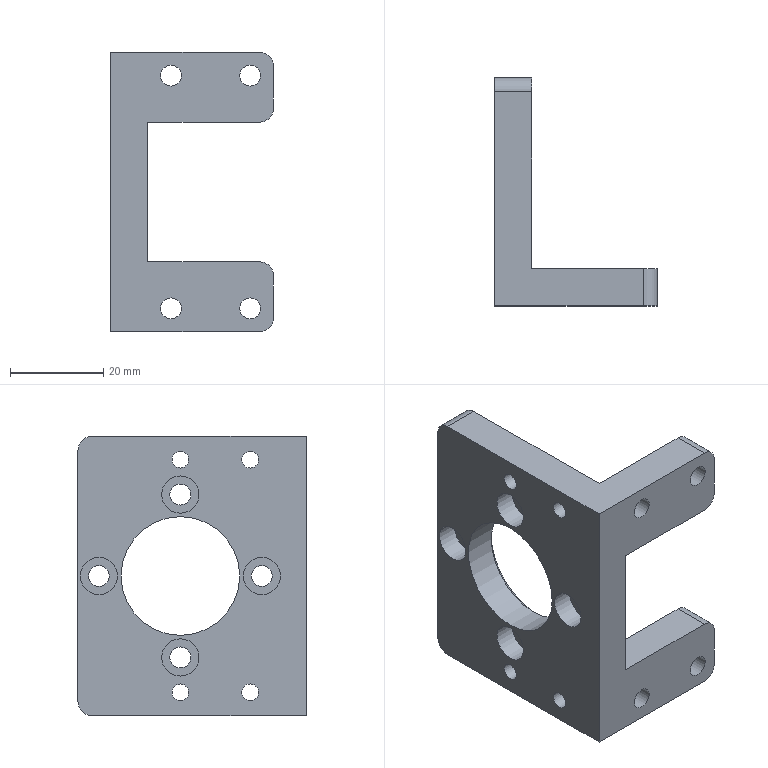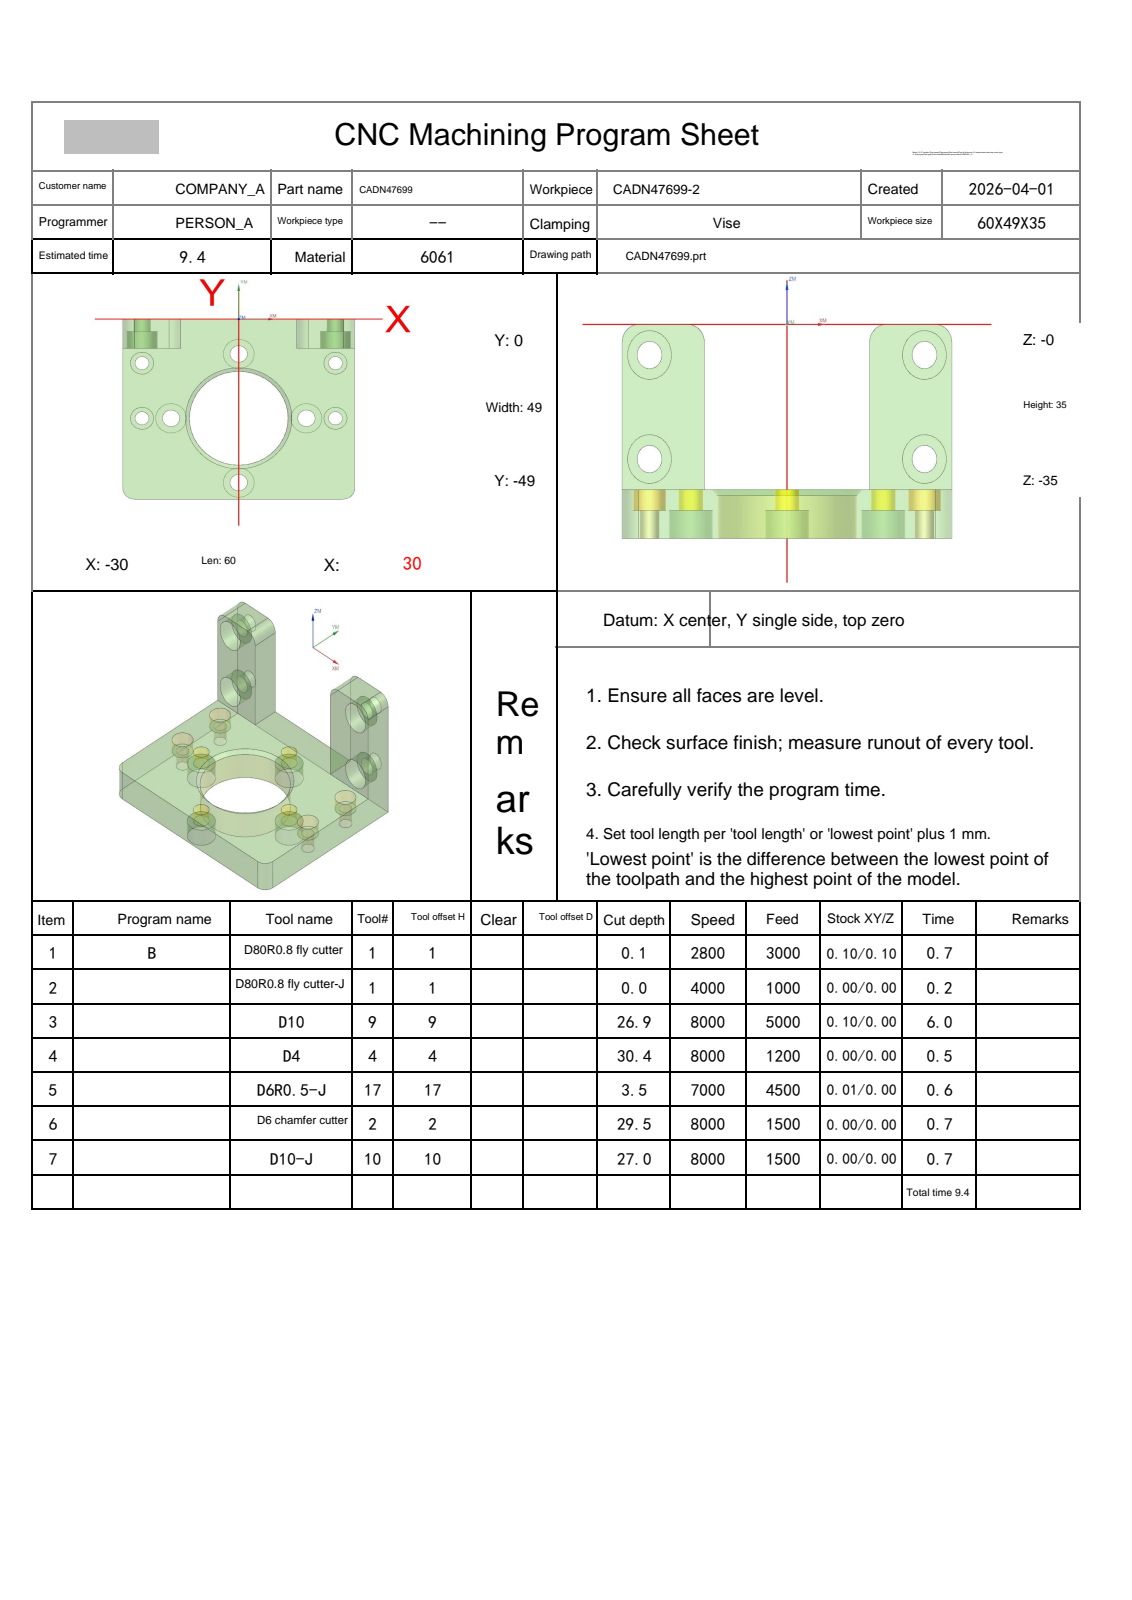NC program | NX | posted by the shop | part box 35 x 49 x 60 mm
Lines 111 to 1367 of 5920:
N3 T09 M06
(D10  D=10. R=0. H=09 ce=0.10 di=0.10)
G00 G90 G54 X0.0 Y-57. M03 S8000
G43 H09 Z14.5
M08
Z.902
G01 Z-.598 F5000.
Y-53.9
X-27.001
G02 X-34.9 Y-46. I.001 J7.9
G01 Y-13.1
X-9.9
Y4.9
X9.9
Y-2.6
Y-13.1
X34.9
Y-46.
G02 X27. Y-53.9 I-7.9 J0.0
G01 X3.035
G02 X2.203 Y-53.455 I0.0 J1.
G01 X-2.203 Y-46.845
G03 X-3.035 Y-46.4 I-.832 J-.555
G01 X-26.402
G02 X-27.4 Y-45.402 I.002 J1.
G01 Y-21.598
G02 X-26.402 Y-20.6 I1. J-.002
G01 X-9.9
G03 X-2.4 Y-13.1 I0.0 J7.5
G01 Y-3.598
G02 X-1.402 Y-2.6 I1. J-.002
G01 X1.402
G02 X2.4 Y-3.598 I-.002 J-1.
G01 Y-13.1
G03 X9.9 Y-20.6 I7.5 J0.0
G01 X26.402
G02 X27.4 Y-21.598 I-.002 J-1.
G01 Y-45.402
G02 X26.402 Y-46.4 I-1. J.002
G01 X3.035
G02 X2.203 Y-45.955 I0.0 J1.
G01 X-2.203 Y-39.345
G03 X-3.035 Y-38.9 I-.832 J-.555
G01 X-18.902
G02 X-19.9 Y-37.902 I.002 J1.
G01 Y-29.098
G02 X-18.902 Y-28.1 I1. J-.002
G01 X-9.9
G03 X-.617 Y-24.882 I0.0 J15.
G02 X0.0 Y-24.669 I.617 J-.787
X.617 Y-24.882 I0.0 J-1.
G03 X9.9 Y-28.1 I9.283 J11.782
G01 X18.902
G02 X19.9 Y-29.098 I-.002 J-1.
G01 Y-37.902
G02 X18.902 Y-38.9 I-1. J.002
G01 X2.664
G02 X1.957 Y-38.607 I0.0 J1.
G01 X-1.957 Y-34.693
G03 X-2.664 Y-34.4 I-.707 J-.707
G01 X-14.502
G02 X-15.4 Y-33.5 I.002 J.9
X-14.502 Y-32.6 I.9 J0.0
G01 X-9.9
G03 X-.481 Y-30.174 I0.0 J19.5
G02 X0.0 Y-30.051 I.481 J-.877
X.481 Y-30.174 I0.0 J-1.
G03 X9.9 Y-32.6 I9.419 J17.074
G01 X14.502
G02 X15.4 Y-33.5 I-.002 J-.9
X14.502 Y-34.4 I-.9 J0.0
G01 X0.0
X-.5
Y-37.4
Z.902
G00 X0.0 Y-57.
Z.304
G01 Z-1.196
Y-53.9
X-27.001
G02 X-34.9 Y-46. I.001 J7.9
G01 Y-13.1
X-9.9
Y4.9
X9.9
Y-2.6
Y-13.1
X34.9
Y-46.
G02 X27. Y-53.9 I-7.9 J0.0
G01 X3.035
G02 X2.203 Y-53.455 I0.0 J1.
G01 X-2.203 Y-46.845
G03 X-3.035 Y-46.4 I-.832 J-.555
G01 X-26.402
G02 X-27.4 Y-45.402 I.002 J1.
G01 Y-21.598
G02 X-26.402 Y-20.6 I1. J-.002
G01 X-9.9
G03 X-2.4 Y-13.1 I0.0 J7.5
G01 Y-3.598
G02 X-1.402 Y-2.6 I1. J-.002
G01 X1.402
G02 X2.4 Y-3.598 I-.002 J-1.
G01 Y-13.1
G03 X9.9 Y-20.6 I7.5 J0.0
G01 X26.402
G02 X27.4 Y-21.598 I-.002 J-1.
G01 Y-45.402
G02 X26.402 Y-46.4 I-1. J.002
G01 X3.035
G02 X2.203 Y-45.955 I0.0 J1.
G01 X-2.203 Y-39.345
G03 X-3.035 Y-38.9 I-.832 J-.555
G01 X-18.902
G02 X-19.9 Y-37.902 I.002 J1.
G01 Y-29.098
G02 X-18.902 Y-28.1 I1. J-.002
G01 X-9.9
G03 X-.617 Y-24.882 I0.0 J15.
G02 X0.0 Y-24.669 I.617 J-.787
X.617 Y-24.882 I0.0 J-1.
G03 X9.9 Y-28.1 I9.283 J11.782
G01 X18.902
G02 X19.9 Y-29.098 I-.002 J-1.
G01 Y-37.902
G02 X18.902 Y-38.9 I-1. J.002
G01 X2.664
G02 X1.957 Y-38.607 I0.0 J1.
G01 X-1.957 Y-34.693
G03 X-2.664 Y-34.4 I-.707 J-.707
G01 X-14.502
G02 X-15.4 Y-33.5 I.002 J.9
X-14.502 Y-32.6 I.9 J0.0
G01 X-9.9
G03 X-.481 Y-30.174 I0.0 J19.5
G02 X0.0 Y-30.051 I.481 J-.877
X.481 Y-30.174 I0.0 J-1.
G03 X9.9 Y-32.6 I9.419 J17.074
G01 X14.502
G02 X15.4 Y-33.5 I-.002 J-.9
X14.502 Y-34.4 I-.9 J0.0
G01 X0.0
X-.5
Y-37.4
Z.304
G00 X0.0 Y-57.
Z-.293
G01 Z-1.793
Y-53.9
X-27.001
G02 X-34.9 Y-46. I.001 J7.9
G01 Y-13.1
X-9.9
Y4.9
X9.9
Y-2.6
Y-13.1
X34.9
Y-46.
G02 X27. Y-53.9 I-7.9 J0.0
G01 X3.035
G02 X2.203 Y-53.455 I0.0 J1.
G01 X-2.203 Y-46.845
G03 X-3.035 Y-46.4 I-.832 J-.555
G01 X-26.402
G02 X-27.4 Y-45.402 I.002 J1.
G01 Y-21.598
G02 X-26.402 Y-20.6 I1. J-.002
G01 X-9.9
G03 X-2.4 Y-13.1 I0.0 J7.5
G01 Y-3.598
G02 X-1.402 Y-2.6 I1. J-.002
G01 X1.402
G02 X2.4 Y-3.598 I-.002 J-1.
G01 Y-13.1
G03 X9.9 Y-20.6 I7.5 J0.0
G01 X26.402
G02 X27.4 Y-21.598 I-.002 J-1.
G01 Y-45.402
G02 X26.402 Y-46.4 I-1. J.002
G01 X3.035
G02 X2.203 Y-45.955 I0.0 J1.
G01 X-2.203 Y-39.345
G03 X-3.035 Y-38.9 I-.832 J-.555
G01 X-18.902
G02 X-19.9 Y-37.902 I.002 J1.
G01 Y-29.098
G02 X-18.902 Y-28.1 I1. J-.002
G01 X-9.9
G03 X-.617 Y-24.882 I0.0 J15.
G02 X0.0 Y-24.669 I.617 J-.787
X.617 Y-24.882 I0.0 J-1.
G03 X9.9 Y-28.1 I9.283 J11.782
G01 X18.902
G02 X19.9 Y-29.098 I-.002 J-1.
G01 Y-37.902
G02 X18.902 Y-38.9 I-1. J.002
G01 X2.664
G02 X1.957 Y-38.607 I0.0 J1.
G01 X-1.957 Y-34.693
G03 X-2.664 Y-34.4 I-.707 J-.707
G01 X-14.502
G02 X-15.4 Y-33.5 I.002 J.9
X-14.502 Y-32.6 I.9 J0.0
G01 X-9.9
G03 X-.481 Y-30.174 I0.0 J19.5
G02 X0.0 Y-30.051 I.481 J-.877
X.481 Y-30.174 I0.0 J-1.
G03 X9.9 Y-32.6 I9.419 J17.074
G01 X14.502
G02 X15.4 Y-33.5 I-.002 J-.9
X14.502 Y-34.4 I-.9 J0.0
G01 X0.0
X-.5
Y-37.4
Z-.293
G00 X0.0 Y-57.
Z-.891
G01 Z-2.391
Y-53.9
X-27.001
G02 X-34.9 Y-46. I.001 J7.9
G01 Y-13.1
X-9.9
Y4.9
X9.9
Y-2.6
Y-13.1
X34.9
Y-46.
G02 X27. Y-53.9 I-7.9 J0.0
G01 X3.035
G02 X2.203 Y-53.455 I0.0 J1.
G01 X-2.203 Y-46.845
G03 X-3.035 Y-46.4 I-.832 J-.555
G01 X-26.402
G02 X-27.4 Y-45.402 I.002 J1.
G01 Y-21.598
G02 X-26.402 Y-20.6 I1. J-.002
G01 X-9.9
G03 X-2.4 Y-13.1 I0.0 J7.5
G01 Y-3.598
G02 X-1.402 Y-2.6 I1. J-.002
G01 X1.402
G02 X2.4 Y-3.598 I-.002 J-1.
G01 Y-13.1
G03 X9.9 Y-20.6 I7.5 J0.0
G01 X26.402
G02 X27.4 Y-21.598 I-.002 J-1.
G01 Y-45.402
G02 X26.402 Y-46.4 I-1. J.002
G01 X3.035
G02 X2.203 Y-45.955 I0.0 J1.
G01 X-2.203 Y-39.345
G03 X-3.035 Y-38.9 I-.832 J-.555
G01 X-18.902
G02 X-19.9 Y-37.902 I.002 J1.
G01 Y-29.098
G02 X-18.902 Y-28.1 I1. J-.002
G01 X-9.9
G03 X-.617 Y-24.882 I0.0 J15.
G02 X0.0 Y-24.669 I.617 J-.787
X.617 Y-24.882 I0.0 J-1.
G03 X9.9 Y-28.1 I9.283 J11.782
G01 X18.902
G02 X19.9 Y-29.098 I-.002 J-1.
G01 Y-37.902
G02 X18.902 Y-38.9 I-1. J.002
G01 X2.664
G02 X1.957 Y-38.607 I0.0 J1.
G01 X-1.957 Y-34.693
G03 X-2.664 Y-34.4 I-.707 J-.707
G01 X-14.502
G02 X-15.4 Y-33.5 I.002 J.9
X-14.502 Y-32.6 I.9 J0.0
G01 X-9.9
G03 X-.481 Y-30.174 I0.0 J19.5
G02 X0.0 Y-30.051 I.481 J-.877
X.481 Y-30.174 I0.0 J-1.
G03 X9.9 Y-32.6 I9.419 J17.074
G01 X14.502
G02 X15.4 Y-33.5 I-.002 J-.9
X14.502 Y-34.4 I-.9 J0.0
G01 X0.0
X-.5
Y-37.4
Z-.891
G00 X0.0 Y-57.
Z-1.489
G01 Z-2.989
Y-53.9
X-27.001
G02 X-34.9 Y-46. I.001 J7.9
G01 Y-13.1
X-9.9
Y4.9
X9.9
Y-2.6
Y-13.1
X34.9
Y-46.
G02 X27. Y-53.9 I-7.9 J0.0
G01 X3.035
G02 X2.203 Y-53.455 I0.0 J1.
G01 X-2.203 Y-46.845
G03 X-3.035 Y-46.4 I-.832 J-.555
G01 X-26.402
G02 X-27.4 Y-45.402 I.002 J1.
G01 Y-21.598
G02 X-26.402 Y-20.6 I1. J-.002
G01 X-9.9
G03 X-2.4 Y-13.1 I0.0 J7.5
G01 Y-3.598
G02 X-1.402 Y-2.6 I1. J-.002
G01 X1.402
G02 X2.4 Y-3.598 I-.002 J-1.
G01 Y-13.1
G03 X9.9 Y-20.6 I7.5 J0.0
G01 X26.402
G02 X27.4 Y-21.598 I-.002 J-1.
G01 Y-45.402
G02 X26.402 Y-46.4 I-1. J.002
G01 X3.035
G02 X2.203 Y-45.955 I0.0 J1.
G01 X-2.203 Y-39.345
G03 X-3.035 Y-38.9 I-.832 J-.555
G01 X-18.902
G02 X-19.9 Y-37.902 I.002 J1.
G01 Y-29.098
G02 X-18.902 Y-28.1 I1. J-.002
G01 X-9.9
G03 X-.617 Y-24.882 I0.0 J15.
G02 X0.0 Y-24.669 I.617 J-.787
X.617 Y-24.882 I0.0 J-1.
G03 X9.9 Y-28.1 I9.283 J11.782
G01 X18.902
G02 X19.9 Y-29.098 I-.002 J-1.
G01 Y-37.902
G02 X18.902 Y-38.9 I-1. J.002
G01 X2.664
G02 X1.957 Y-38.607 I0.0 J1.
G01 X-1.957 Y-34.693
G03 X-2.664 Y-34.4 I-.707 J-.707
G01 X-14.502
G02 X-15.4 Y-33.5 I.002 J.9
X-14.502 Y-32.6 I.9 J0.0
G01 X-9.9
G03 X-.481 Y-30.174 I0.0 J19.5
G02 X0.0 Y-30.051 I.481 J-.877
X.481 Y-30.174 I0.0 J-1.
G03 X9.9 Y-32.6 I9.419 J17.074
G01 X14.502
G02 X15.4 Y-33.5 I-.002 J-.9
X14.502 Y-34.4 I-.9 J0.0
G01 X0.0
X-.5
Y-37.4
Z-1.489
G00 X0.0 Y-57.
Z-2.087
G01 Z-3.587
Y-53.9
X-27.001
G02 X-34.9 Y-46. I.001 J7.9
G01 Y-13.1
X-9.9
Y4.9
X9.9
Y-2.6
Y-13.1
X34.9
Y-46.
G02 X27. Y-53.9 I-7.9 J0.0
G01 X3.035
G02 X2.203 Y-53.455 I0.0 J1.
G01 X-2.203 Y-46.845
G03 X-3.035 Y-46.4 I-.832 J-.555
G01 X-26.402
G02 X-27.4 Y-45.402 I.002 J1.
G01 Y-21.598
G02 X-26.402 Y-20.6 I1. J-.002
G01 X-9.9
G03 X-2.4 Y-13.1 I0.0 J7.5
G01 Y-3.598
G02 X-1.402 Y-2.6 I1. J-.002
G01 X1.402
G02 X2.4 Y-3.598 I-.002 J-1.
G01 Y-13.1
G03 X9.9 Y-20.6 I7.5 J0.0
G01 X26.402
G02 X27.4 Y-21.598 I-.002 J-1.
G01 Y-45.402
G02 X26.402 Y-46.4 I-1. J.002
G01 X3.035
G02 X2.203 Y-45.955 I0.0 J1.
G01 X-2.203 Y-39.345
G03 X-3.035 Y-38.9 I-.832 J-.555
G01 X-18.902
G02 X-19.9 Y-37.902 I.002 J1.
G01 Y-29.098
G02 X-18.902 Y-28.1 I1. J-.002
G01 X-9.9
G03 X-.617 Y-24.882 I0.0 J15.
G02 X0.0 Y-24.669 I.617 J-.787
X.617 Y-24.882 I0.0 J-1.
G03 X9.9 Y-28.1 I9.283 J11.782
G01 X18.902
G02 X19.9 Y-29.098 I-.002 J-1.
G01 Y-37.902
G02 X18.902 Y-38.9 I-1. J.002
G01 X2.664
G02 X1.957 Y-38.607 I0.0 J1.
G01 X-1.957 Y-34.693
G03 X-2.664 Y-34.4 I-.707 J-.707
G01 X-14.502
G02 X-15.4 Y-33.5 I.002 J.9
X-14.502 Y-32.6 I.9 J0.0
G01 X-9.9
G03 X-.481 Y-30.174 I0.0 J19.5
G02 X0.0 Y-30.051 I.481 J-.877
X.481 Y-30.174 I0.0 J-1.
G03 X9.9 Y-32.6 I9.419 J17.074
G01 X14.502
G02 X15.4 Y-33.5 I-.002 J-.9
X14.502 Y-34.4 I-.9 J0.0
G01 X0.0
X-.5
Y-37.4
Z-2.087
G00 X0.0 Y-57.
Z-2.684
G01 Z-4.184
Y-53.9
X-27.001
G02 X-34.9 Y-46. I.001 J7.9
G01 Y-13.1
X-9.9
Y4.9
X9.9
Y-2.6
Y-13.1
X34.9
Y-46.
G02 X27. Y-53.9 I-7.9 J0.0
G01 X3.035
G02 X2.203 Y-53.455 I0.0 J1.
G01 X-2.203 Y-46.845
G03 X-3.035 Y-46.4 I-.832 J-.555
G01 X-26.402
G02 X-27.4 Y-45.402 I.002 J1.
G01 Y-21.598
G02 X-26.402 Y-20.6 I1. J-.002
G01 X-9.9
G03 X-2.4 Y-13.1 I0.0 J7.5
G01 Y-3.598
G02 X-1.402 Y-2.6 I1. J-.002
G01 X1.402
G02 X2.4 Y-3.598 I-.002 J-1.
G01 Y-13.1
G03 X9.9 Y-20.6 I7.5 J0.0
G01 X26.402
G02 X27.4 Y-21.598 I-.002 J-1.
G01 Y-45.402
G02 X26.402 Y-46.4 I-1. J.002
G01 X3.035
G02 X2.203 Y-45.955 I0.0 J1.
G01 X-2.203 Y-39.345
G03 X-3.035 Y-38.9 I-.832 J-.555
G01 X-18.902
G02 X-19.9 Y-37.902 I.002 J1.
G01 Y-29.098
G02 X-18.902 Y-28.1 I1. J-.002
G01 X-9.9
G03 X-.617 Y-24.882 I0.0 J15.
G02 X0.0 Y-24.669 I.617 J-.787
X.617 Y-24.882 I0.0 J-1.
G03 X9.9 Y-28.1 I9.283 J11.782
G01 X18.902
G02 X19.9 Y-29.098 I-.002 J-1.
G01 Y-37.902
G02 X18.902 Y-38.9 I-1. J.002
G01 X2.664
G02 X1.957 Y-38.607 I0.0 J1.
G01 X-1.957 Y-34.693
G03 X-2.664 Y-34.4 I-.707 J-.707
G01 X-14.502
G02 X-15.4 Y-33.5 I.002 J.9
X-14.502 Y-32.6 I.9 J0.0
G01 X-9.9
G03 X-.481 Y-30.174 I0.0 J19.5
G02 X0.0 Y-30.051 I.481 J-.877
X.481 Y-30.174 I0.0 J-1.
G03 X9.9 Y-32.6 I9.419 J17.074
G01 X14.502
G02 X15.4 Y-33.5 I-.002 J-.9
X14.502 Y-34.4 I-.9 J0.0
G01 X0.0
X-.5
Y-37.4
Z-2.684
G00 X0.0 Y-57.
Z-3.282
G01 Z-4.782
Y-53.9
X-27.001
G02 X-34.9 Y-46. I.001 J7.9
G01 Y-13.1
X-9.9
Y4.9
X9.9
Y-2.6
Y-13.1
X34.9
Y-46.
G02 X27. Y-53.9 I-7.9 J0.0
G01 X3.035
G02 X2.203 Y-53.455 I0.0 J1.
G01 X-2.203 Y-46.845
G03 X-3.035 Y-46.4 I-.832 J-.555
G01 X-26.402
G02 X-27.4 Y-45.402 I.002 J1.
G01 Y-21.598
G02 X-26.402 Y-20.6 I1. J-.002
G01 X-9.9
G03 X-2.4 Y-13.1 I0.0 J7.5
G01 Y-3.598
G02 X-1.402 Y-2.6 I1. J-.002
G01 X1.402
G02 X2.4 Y-3.598 I-.002 J-1.
G01 Y-13.1
G03 X9.9 Y-20.6 I7.5 J0.0
G01 X26.402
G02 X27.4 Y-21.598 I-.002 J-1.
G01 Y-45.402
G02 X26.402 Y-46.4 I-1. J.002
G01 X3.035
G02 X2.203 Y-45.955 I0.0 J1.
G01 X-2.203 Y-39.345
G03 X-3.035 Y-38.9 I-.832 J-.555
G01 X-18.902
G02 X-19.9 Y-37.902 I.002 J1.
G01 Y-29.098
G02 X-18.902 Y-28.1 I1. J-.002
G01 X-9.9
G03 X-.617 Y-24.882 I0.0 J15.
G02 X0.0 Y-24.669 I.617 J-.787
X.617 Y-24.882 I0.0 J-1.
G03 X9.9 Y-28.1 I9.283 J11.782
G01 X18.902
G02 X19.9 Y-29.098 I-.002 J-1.
G01 Y-37.902
G02 X18.902 Y-38.9 I-1. J.002
G01 X2.664
G02 X1.957 Y-38.607 I0.0 J1.
G01 X-1.957 Y-34.693
G03 X-2.664 Y-34.4 I-.707 J-.707
G01 X-14.502
G02 X-15.4 Y-33.5 I.002 J.9
X-14.502 Y-32.6 I.9 J0.0
G01 X-9.9
G03 X-.481 Y-30.174 I0.0 J19.5
G02 X0.0 Y-30.051 I.481 J-.877
X.481 Y-30.174 I0.0 J-1.
G03 X9.9 Y-32.6 I9.419 J17.074
G01 X14.502
G02 X15.4 Y-33.5 I-.002 J-.9
X14.502 Y-34.4 I-.9 J0.0
G01 X0.0
X-.5
Y-37.4
Z-3.282
G00 X0.0 Y-57.
Z-3.88
G01 Z-5.38
Y-53.9
X-27.001
G02 X-34.9 Y-46. I.001 J7.9
G01 Y-13.1
X-9.9
Y4.9
X9.9
Y-2.6
Y-13.1
X34.9
Y-46.
G02 X27. Y-53.9 I-7.9 J0.0
G01 X3.035
G02 X2.203 Y-53.455 I0.0 J1.
G01 X-2.203 Y-46.845
G03 X-3.035 Y-46.4 I-.832 J-.555
G01 X-26.402
G02 X-27.4 Y-45.402 I.002 J1.
G01 Y-21.598
G02 X-26.402 Y-20.6 I1. J-.002
G01 X-9.9
G03 X-2.4 Y-13.1 I0.0 J7.5
G01 Y-3.598
G02 X-1.402 Y-2.6 I1. J-.002
G01 X1.402
G02 X2.4 Y-3.598 I-.002 J-1.
G01 Y-13.1
G03 X9.9 Y-20.6 I7.5 J0.0
G01 X26.402
G02 X27.4 Y-21.598 I-.002 J-1.
G01 Y-45.402
G02 X26.402 Y-46.4 I-1. J.002
G01 X3.035
G02 X2.203 Y-45.955 I0.0 J1.
G01 X-2.203 Y-39.345
G03 X-3.035 Y-38.9 I-.832 J-.555
G01 X-18.902
G02 X-19.9 Y-37.902 I.002 J1.
G01 Y-29.098
G02 X-18.902 Y-28.1 I1. J-.002
G01 X-9.9
G03 X-.617 Y-24.882 I0.0 J15.
G02 X0.0 Y-24.669 I.617 J-.787
X.617 Y-24.882 I0.0 J-1.
G03 X9.9 Y-28.1 I9.283 J11.782
G01 X18.902
G02 X19.9 Y-29.098 I-.002 J-1.
G01 Y-37.902
G02 X18.902 Y-38.9 I-1. J.002
G01 X2.664
G02 X1.957 Y-38.607 I0.0 J1.
G01 X-1.957 Y-34.693
G03 X-2.664 Y-34.4 I-.707 J-.707
G01 X-14.502
G02 X-15.4 Y-33.5 I.002 J.9
X-14.502 Y-32.6 I.9 J0.0
G01 X-9.9
G03 X-.481 Y-30.174 I0.0 J19.5
G02 X0.0 Y-30.051 I.481 J-.877
X.481 Y-30.174 I0.0 J-1.
G03 X9.9 Y-32.6 I9.419 J17.074
G01 X14.502
G02 X15.4 Y-33.5 I-.002 J-.9
X14.502 Y-34.4 I-.9 J0.0
G01 X0.0
X-.5
Y-37.4
Z-3.88
G00 X0.0 Y-57.
Z-4.478
G01 Z-5.978
Y-53.9
X-27.001
G02 X-34.9 Y-46. I.001 J7.9
G01 Y-13.1
X-9.9
Y4.9
X9.9
Y-2.6
Y-13.1
X34.9
Y-46.
G02 X27. Y-53.9 I-7.9 J0.0
G01 X3.035
G02 X2.203 Y-53.455 I0.0 J1.
G01 X-2.203 Y-46.845
G03 X-3.035 Y-46.4 I-.832 J-.555
G01 X-26.402
G02 X-27.4 Y-45.402 I.002 J1.
G01 Y-21.598
G02 X-26.402 Y-20.6 I1. J-.002
G01 X-9.9
G03 X-2.4 Y-13.1 I0.0 J7.5
G01 Y-3.598
G02 X-1.402 Y-2.6 I1. J-.002
G01 X1.402
G02 X2.4 Y-3.598 I-.002 J-1.
G01 Y-13.1
G03 X9.9 Y-20.6 I7.5 J0.0
G01 X26.402
G02 X27.4 Y-21.598 I-.002 J-1.
G01 Y-45.402
G02 X26.402 Y-46.4 I-1. J.002
G01 X3.035
G02 X2.203 Y-45.955 I0.0 J1.
G01 X-2.203 Y-39.345
G03 X-3.035 Y-38.9 I-.832 J-.555
G01 X-18.902
G02 X-19.9 Y-37.902 I.002 J1.
G01 Y-29.098
G02 X-18.902 Y-28.1 I1. J-.002
G01 X-9.9
G03 X-.617 Y-24.882 I0.0 J15.
G02 X0.0 Y-24.669 I.617 J-.787
X.617 Y-24.882 I0.0 J-1.
G03 X9.9 Y-28.1 I9.283 J11.782
G01 X18.902
G02 X19.9 Y-29.098 I-.002 J-1.
G01 Y-37.902
G02 X18.902 Y-38.9 I-1. J.002
G01 X2.664
G02 X1.957 Y-38.607 I0.0 J1.
G01 X-1.957 Y-34.693
G03 X-2.664 Y-34.4 I-.707 J-.707
G01 X-14.502
G02 X-15.4 Y-33.5 I.002 J.9
X-14.502 Y-32.6 I.9 J0.0
G01 X-9.9
G03 X-.481 Y-30.174 I0.0 J19.5
G02 X0.0 Y-30.051 I.481 J-.877
X.481 Y-30.174 I0.0 J-1.
G03 X9.9 Y-32.6 I9.419 J17.074
G01 X14.502
G02 X15.4 Y-33.5 I-.002 J-.9
X14.502 Y-34.4 I-.9 J0.0
G01 X0.0
X-.5
Y-37.4
Z-4.478
G00 X0.0 Y-57.
Z-5.076
G01 Z-6.576
Y-53.9
X-27.001
G02 X-34.9 Y-46. I.001 J7.9
G01 Y-13.1
X-9.9
Y4.9
X9.9
Y-2.6
Y-13.1
X34.9
Y-46.
G02 X27. Y-53.9 I-7.9 J0.0
G01 X3.035
G02 X2.203 Y-53.455 I0.0 J1.
G01 X-2.203 Y-46.845
G03 X-3.035 Y-46.4 I-.832 J-.555
G01 X-26.402
G02 X-27.4 Y-45.402 I.002 J1.
G01 Y-21.598
G02 X-26.402 Y-20.6 I1. J-.002
G01 X-9.9
G03 X-2.4 Y-13.1 I0.0 J7.5
G01 Y-3.598
G02 X-1.402 Y-2.6 I1. J-.002
G01 X1.402
G02 X2.4 Y-3.598 I-.002 J-1.
G01 Y-13.1
G03 X9.9 Y-20.6 I7.5 J0.0
G01 X26.402
G02 X27.4 Y-21.598 I-.002 J-1.
G01 Y-45.402
G02 X26.402 Y-46.4 I-1. J.002
G01 X3.035
G02 X2.203 Y-45.955 I0.0 J1.
G01 X-2.203 Y-39.345
G03 X-3.035 Y-38.9 I-.832 J-.555
G01 X-18.902
G02 X-19.9 Y-37.902 I.002 J1.
G01 Y-29.098
G02 X-18.902 Y-28.1 I1. J-.002
G01 X-9.9
G03 X-.617 Y-24.882 I0.0 J15.
G02 X0.0 Y-24.669 I.617 J-.787
X.617 Y-24.882 I0.0 J-1.
G03 X9.9 Y-28.1 I9.283 J11.782
G01 X18.902
G02 X19.9 Y-29.098 I-.002 J-1.
G01 Y-37.902
G02 X18.902 Y-38.9 I-1. J.002
G01 X2.664
G02 X1.957 Y-38.607 I0.0 J1.
G01 X-1.957 Y-34.693
G03 X-2.664 Y-34.4 I-.707 J-.707
G01 X-14.502
G02 X-15.4 Y-33.5 I.002 J.9
X-14.502 Y-32.6 I.9 J0.0
G01 X-9.9
G03 X-.481 Y-30.174 I0.0 J19.5
G02 X0.0 Y-30.051 I.481 J-.877
X.481 Y-30.174 I0.0 J-1.
G03 X9.9 Y-32.6 I9.419 J17.074
G01 X14.502
G02 X15.4 Y-33.5 I-.002 J-.9
X14.502 Y-34.4 I-.9 J0.0
G01 X0.0
X-.5
Y-37.4
Z-5.076
G00 X0.0 Y-57.
Z-5.673
G01 Z-7.173
Y-53.9
X-27.001
G02 X-34.9 Y-46. I.001 J7.9
G01 Y-13.1
X-9.9
Y4.9
X9.9
Y-2.6
Y-13.1
X34.9
Y-46.
G02 X27. Y-53.9 I-7.9 J0.0
G01 X3.035
G02 X2.203 Y-53.455 I0.0 J1.
G01 X-2.203 Y-46.845
G03 X-3.035 Y-46.4 I-.832 J-.555
G01 X-26.402
G02 X-27.4 Y-45.402 I.002 J1.
G01 Y-21.598
G02 X-26.402 Y-20.6 I1. J-.002
G01 X-9.9
G03 X-2.4 Y-13.1 I0.0 J7.5
G01 Y-3.598
G02 X-1.402 Y-2.6 I1. J-.002
G01 X1.402
G02 X2.4 Y-3.598 I-.002 J-1.
G01 Y-13.1
G03 X9.9 Y-20.6 I7.5 J0.0
G01 X26.402
G02 X27.4 Y-21.598 I-.002 J-1.
G01 Y-45.402
G02 X26.402 Y-46.4 I-1. J.002
G01 X3.035
G02 X2.203 Y-45.955 I0.0 J1.
G01 X-2.203 Y-39.345
G03 X-3.035 Y-38.9 I-.832 J-.555
G01 X-18.902
G02 X-19.9 Y-37.902 I.002 J1.
G01 Y-29.098
G02 X-18.902 Y-28.1 I1. J-.002
G01 X-9.9
G03 X-.617 Y-24.882 I0.0 J15.
G02 X0.0 Y-24.669 I.617 J-.787
X.617 Y-24.882 I0.0 J-1.
G03 X9.9 Y-28.1 I9.283 J11.782
G01 X18.902
G02 X19.9 Y-29.098 I-.002 J-1.
G01 Y-37.902
G02 X18.902 Y-38.9 I-1. J.002
G01 X2.664
G02 X1.957 Y-38.607 I0.0 J1.
G01 X-1.957 Y-34.693
G03 X-2.664 Y-34.4 I-.707 J-.707
G01 X-14.502
G02 X-15.4 Y-33.5 I.002 J.9
X-14.502 Y-32.6 I.9 J0.0
G01 X-9.9
G03 X-.481 Y-30.174 I0.0 J19.5
G02 X0.0 Y-30.051 I.481 J-.877
X.481 Y-30.174 I0.0 J-1.
G03 X9.9 Y-32.6 I9.419 J17.074
G01 X14.502
G02 X15.4 Y-33.5 I-.002 J-.9
X14.502 Y-34.4 I-.9 J0.0
G01 X0.0
X-.5
Y-37.4
Z-5.673
G00 X0.0 Y-57.
Z-6.271
G01 Z-7.771
Y-53.9
X-27.001
G02 X-34.9 Y-46. I.001 J7.9
G01 Y-13.1
X-9.9
Y4.9
X9.9
Y-2.6
Y-13.1
X34.9
Y-46.
G02 X27. Y-53.9 I-7.9 J0.0
G01 X3.035
G02 X2.203 Y-53.455 I0.0 J1.
G01 X-2.203 Y-46.845
G03 X-3.035 Y-46.4 I-.832 J-.555
G01 X-26.402
G02 X-27.4 Y-45.402 I.002 J1.
G01 Y-21.598
G02 X-26.402 Y-20.6 I1. J-.002
G01 X-9.9
G03 X-2.4 Y-13.1 I0.0 J7.5
G01 Y-3.598
G02 X-1.402 Y-2.6 I1. J-.002
G01 X1.402
G02 X2.4 Y-3.598 I-.002 J-1.
G01 Y-13.1
G03 X9.9 Y-20.6 I7.5 J0.0
G01 X26.402
G02 X27.4 Y-21.598 I-.002 J-1.
G01 Y-45.402
G02 X26.402 Y-46.4 I-1. J.002
G01 X3.035
G02 X2.203 Y-45.955 I0.0 J1.
G01 X-2.203 Y-39.345
G03 X-3.035 Y-38.9 I-.832 J-.555
G01 X-18.902
G02 X-19.9 Y-37.902 I.002 J1.
G01 Y-29.098
G02 X-18.902 Y-28.1 I1. J-.002
G01 X-9.9
G03 X-.617 Y-24.882 I0.0 J15.
G02 X0.0 Y-24.669 I.617 J-.787
X.617 Y-24.882 I0.0 J-1.
G03 X9.9 Y-28.1 I9.283 J11.782
G01 X18.902
G02 X19.9 Y-29.098 I-.002 J-1.
G01 Y-37.902
G02 X18.902 Y-38.9 I-1. J.002
G01 X2.664
G02 X1.957 Y-38.607 I0.0 J1.
G01 X-1.957 Y-34.693
G03 X-2.664 Y-34.4 I-.707 J-.707
G01 X-14.502
G02 X-15.4 Y-33.5 I.002 J.9
X-14.502 Y-32.6 I.9 J0.0
G01 X-9.9
G03 X-.481 Y-30.174 I0.0 J19.5
G02 X0.0 Y-30.051 I.481 J-.877
X.481 Y-30.174 I0.0 J-1.
G03 X9.9 Y-32.6 I9.419 J17.074
G01 X14.502
G02 X15.4 Y-33.5 I-.002 J-.9
X14.502 Y-34.4 I-.9 J0.0
G01 X0.0
X-.5
Y-37.4
Z-6.271
G00 X0.0 Y-57.
Z-6.869
G01 Z-8.369
Y-53.9
X-27.001
G02 X-34.9 Y-46. I.001 J7.9
G01 Y-13.1
X-9.9
Y4.9
X9.9
Y-2.6
Y-13.1
X34.9
Y-46.
G02 X27. Y-53.9 I-7.9 J0.0
G01 X3.035
G02 X2.203 Y-53.455 I0.0 J1.
G01 X-2.203 Y-46.845
G03 X-3.035 Y-46.4 I-.832 J-.555
G01 X-26.402
G02 X-27.4 Y-45.402 I.002 J1.
G01 Y-21.598
G02 X-26.402 Y-20.6 I1. J-.002
G01 X-9.9
G03 X-2.4 Y-13.1 I0.0 J7.5
G01 Y-3.598
G02 X-1.402 Y-2.6 I1. J-.002
G01 X1.402
G02 X2.4 Y-3.598 I-.002 J-1.
G01 Y-13.1
G03 X9.9 Y-20.6 I7.5 J0.0
G01 X26.402
G02 X27.4 Y-21.598 I-.002 J-1.
G01 Y-45.402
G02 X26.402 Y-46.4 I-1. J.002
G01 X3.035
G02 X2.203 Y-45.955 I0.0 J1.
G01 X-2.203 Y-39.345
G03 X-3.035 Y-38.9 I-.832 J-.555
G01 X-18.902
G02 X-19.9 Y-37.902 I.002 J1.
G01 Y-29.098
G02 X-18.902 Y-28.1 I1. J-.002
G01 X-9.9
G03 X-.617 Y-24.882 I0.0 J15.
G02 X0.0 Y-24.669 I.617 J-.787
X.617 Y-24.882 I0.0 J-1.
G03 X9.9 Y-28.1 I9.283 J11.782
G01 X18.902
G02 X19.9 Y-29.098 I-.002 J-1.
G01 Y-37.902
G02 X18.902 Y-38.9 I-1. J.002
G01 X2.664
G02 X1.957 Y-38.607 I0.0 J1.
G01 X-1.957 Y-34.693
G03 X-2.664 Y-34.4 I-.707 J-.707
G01 X-14.502
G02 X-15.4 Y-33.5 I.002 J.9
X-14.502 Y-32.6 I.9 J0.0
G01 X-9.9
G03 X-.481 Y-30.174 I0.0 J19.5
G02 X0.0 Y-30.051 I.481 J-.877
X.481 Y-30.174 I0.0 J-1.
G03 X9.9 Y-32.6 I9.419 J17.074
G01 X14.502
G02 X15.4 Y-33.5 I-.002 J-.9
X14.502 Y-34.4 I-.9 J0.0
G01 X0.0
X-.5
Y-37.4
Z-6.869
G00 X0.0 Y-57.
Z-7.467
G01 Z-8.967
Y-53.9
X-27.001
G02 X-34.9 Y-46. I.001 J7.9
G01 Y-13.1
X-9.9
Y4.9
X9.9
Y-2.6
Y-13.1
X34.9
Y-46.
G02 X27. Y-53.9 I-7.9 J0.0
G01 X3.035
G02 X2.203 Y-53.455 I0.0 J1.
G01 X-2.203 Y-46.845
G03 X-3.035 Y-46.4 I-.832 J-.555
G01 X-26.402
G02 X-27.4 Y-45.402 I.002 J1.
G01 Y-21.598
G02 X-26.402 Y-20.6 I1. J-.002
G01 X-9.9
G03 X-2.4 Y-13.1 I0.0 J7.5
G01 Y-3.598
G02 X-1.402 Y-2.6 I1. J-.002
G01 X1.402
G02 X2.4 Y-3.598 I-.002 J-1.
G01 Y-13.1
G03 X9.9 Y-20.6 I7.5 J0.0
G01 X26.402
G02 X27.4 Y-21.598 I-.002 J-1.
G01 Y-45.402
G02 X26.402 Y-46.4 I-1. J.002
G01 X3.035
G02 X2.203 Y-45.955 I0.0 J1.
G01 X-2.203 Y-39.345
G03 X-3.035 Y-38.9 I-.832 J-.555
G01 X-18.902
G02 X-19.9 Y-37.902 I.002 J1.
G01 Y-29.098
G02 X-18.902 Y-28.1 I1. J-.002
G01 X-9.9
G03 X-.617 Y-24.882 I0.0 J15.
G02 X0.0 Y-24.669 I.617 J-.787
X.617 Y-24.882 I0.0 J-1.
G03 X9.9 Y-28.1 I9.283 J11.782
G01 X18.902
G02 X19.9 Y-29.098 I-.002 J-1.
G01 Y-37.902
G02 X18.902 Y-38.9 I-1. J.002
G01 X2.664
G02 X1.957 Y-38.607 I0.0 J1.
G01 X-1.957 Y-34.693
G03 X-2.664 Y-34.4 I-.707 J-.707
G01 X-14.502
G02 X-15.4 Y-33.5 I.002 J.9
X-14.502 Y-32.6 I.9 J0.0
G01 X-9.9
G03 X-.481 Y-30.174 I0.0 J19.5
G02 X0.0 Y-30.051 I.481 J-.877
X.481 Y-30.174 I0.0 J-1.
G03 X9.9 Y-32.6 I9.419 J17.074
G01 X14.502
G02 X15.4 Y-33.5 I-.002 J-.9
X14.502 Y-34.4 I-.9 J0.0
G01 X0.0
X-.5
Y-37.4
Z-7.467
G00 X0.0 Y-57.
Z-8.064
G01 Z-9.564
Y-53.9
X-27.001
G02 X-34.9 Y-46. I.001 J7.9
G01 Y-13.1
X-9.9
Y4.9
X9.9
Y-2.6
Y-13.1
X34.9
Y-46.
G02 X27. Y-53.9 I-7.9 J0.0
G01 X3.035
G02 X2.203 Y-53.455 I0.0 J1.
G01 X-2.203 Y-46.845
G03 X-3.035 Y-46.4 I-.832 J-.555
G01 X-26.402
G02 X-27.4 Y-45.402 I.002 J1.
G01 Y-21.598
G02 X-26.402 Y-20.6 I1. J-.002
G01 X-9.9
G03 X-2.4 Y-13.1 I0.0 J7.5
G01 Y-3.598
G02 X-1.402 Y-2.6 I1. J-.002
G01 X1.402
G02 X2.4 Y-3.598 I-.002 J-1.
G01 Y-13.1
G03 X9.9 Y-20.6 I7.5 J0.0
G01 X26.402
G02 X27.4 Y-21.598 I-.002 J-1.
G01 Y-45.402
G02 X26.402 Y-46.4 I-1. J.002
G01 X3.035
G02 X2.203 Y-45.955 I0.0 J1.
G01 X-2.203 Y-39.345
G03 X-3.035 Y-38.9 I-.832 J-.555
G01 X-18.902
G02 X-19.9 Y-37.902 I.002 J1.
G01 Y-29.098
G02 X-18.902 Y-28.1 I1. J-.002
G01 X-9.9
G03 X-.617 Y-24.882 I0.0 J15.
G02 X0.0 Y-24.669 I.617 J-.787
X.617 Y-24.882 I0.0 J-1.
G03 X9.9 Y-28.1 I9.283 J11.782
G01 X18.902
G02 X19.9 Y-29.098 I-.002 J-1.
G01 Y-37.902
G02 X18.902 Y-38.9 I-1. J.002
G01 X2.664
G02 X1.957 Y-38.607 I0.0 J1.
G01 X-1.957 Y-34.693
G03 X-2.664 Y-34.4 I-.707 J-.707
G01 X-14.502
G02 X-15.4 Y-33.5 I.002 J.9
X-14.502 Y-32.6 I.9 J0.0
G01 X-9.9
G03 X-.481 Y-30.174 I0.0 J19.5
G02 X0.0 Y-30.051 I.481 J-.877
X.481 Y-30.174 I0.0 J-1.
G03 X9.9 Y-32.6 I9.419 J17.074
G01 X14.502
G02 X15.4 Y-33.5 I-.002 J-.9
X14.502 Y-34.4 I-.9 J0.0
G01 X0.0
X-.5
Y-37.4
Z-8.064
G00 X0.0 Y-57.
Z-8.662
G01 Z-10.162
Y-53.9
X-27.001
G02 X-34.9 Y-46. I.001 J7.9
G01 Y-13.1
X-9.9
Y4.9
X9.9
Y-2.6
Y-13.1
X34.9
Y-46.
G02 X27. Y-53.9 I-7.9 J0.0
G01 X3.035
G02 X2.203 Y-53.455 I0.0 J1.
G01 X-2.203 Y-46.845
G03 X-3.035 Y-46.4 I-.832 J-.555
G01 X-26.402
G02 X-27.4 Y-45.402 I.002 J1.
G01 Y-21.598
G02 X-26.402 Y-20.6 I1. J-.002
G01 X-9.9
G03 X-2.4 Y-13.1 I0.0 J7.5
G01 Y-3.598
G02 X-1.402 Y-2.6 I1. J-.002
G01 X1.402
G02 X2.4 Y-3.598 I-.002 J-1.
G01 Y-13.1
G03 X9.9 Y-20.6 I7.5 J0.0
G01 X26.402
G02 X27.4 Y-21.598 I-.002 J-1.
G01 Y-45.402
G02 X26.402 Y-46.4 I-1. J.002
G01 X3.035
G02 X2.203 Y-45.955 I0.0 J1.
G01 X-2.203 Y-39.345
G03 X-3.035 Y-38.9 I-.832 J-.555
G01 X-18.902
G02 X-19.9 Y-37.902 I.002 J1.
G01 Y-29.098
G02 X-18.902 Y-28.1 I1. J-.002
G01 X-9.9
G03 X-.617 Y-24.882 I0.0 J15.
G02 X0.0 Y-24.669 I.617 J-.787
X.617 Y-24.882 I0.0 J-1.
G03 X9.9 Y-28.1 I9.283 J11.782
G01 X18.902
G02 X19.9 Y-29.098 I-.002 J-1.
G01 Y-37.902
G02 X18.902 Y-38.9 I-1. J.002
G01 X2.664
G02 X1.957 Y-38.607 I0.0 J1.
G01 X-1.957 Y-34.693
G03 X-2.664 Y-34.4 I-.707 J-.707
G01 X-14.502
G02 X-15.4 Y-33.5 I.002 J.9
X-14.502 Y-32.6 I.9 J0.0
G01 X-9.9
G03 X-.481 Y-30.174 I0.0 J19.5
G02 X0.0 Y-30.051 I.481 J-.877
X.481 Y-30.174 I0.0 J-1.
G03 X9.9 Y-32.6 I9.419 J17.074
G01 X14.502
G02 X15.4 Y-33.5 I-.002 J-.9
X14.502 Y-34.4 I-.9 J0.0
G01 X0.0
X-.5
Y-37.4
Z-8.662
G00 X0.0 Y-57.
Z-9.26
G01 Z-10.76
Y-53.9
X-27.001
G02 X-34.9 Y-46. I.001 J7.9
G01 Y-13.1
X-9.9
Y4.9
X9.9
Y-2.6
Y-13.1
X34.9
Y-46.
G02 X27. Y-53.9 I-7.9 J0.0
G01 X3.035
G02 X2.203 Y-53.455 I0.0 J1.
G01 X-2.203 Y-46.845
G03 X-3.035 Y-46.4 I-.832 J-.555
G01 X-26.402
G02 X-27.4 Y-45.402 I.002 J1.
G01 Y-21.598
G02 X-26.402 Y-20.6 I1. J-.002
G01 X-9.9
G03 X-2.4 Y-13.1 I0.0 J7.5
G01 Y-3.598
G02 X-1.402 Y-2.6 I1. J-.002
G01 X1.402
G02 X2.4 Y-3.598 I-.002 J-1.
G01 Y-13.1
G03 X9.9 Y-20.6 I7.5 J0.0
G01 X26.402
G02 X27.4 Y-21.598 I-.002 J-1.
G01 Y-45.402
G02 X26.402 Y-46.4 I-1. J.002
G01 X3.035
G02 X2.203 Y-45.955 I0.0 J1.
G01 X-2.203 Y-39.345
G03 X-3.035 Y-38.9 I-.832 J-.555
G01 X-18.902
G02 X-19.9 Y-37.902 I.002 J1.
G01 Y-29.098
G02 X-18.902 Y-28.1 I1. J-.002
G01 X-9.9
G03 X-.617 Y-24.882 I0.0 J15.
G02 X0.0 Y-24.669 I.617 J-.787